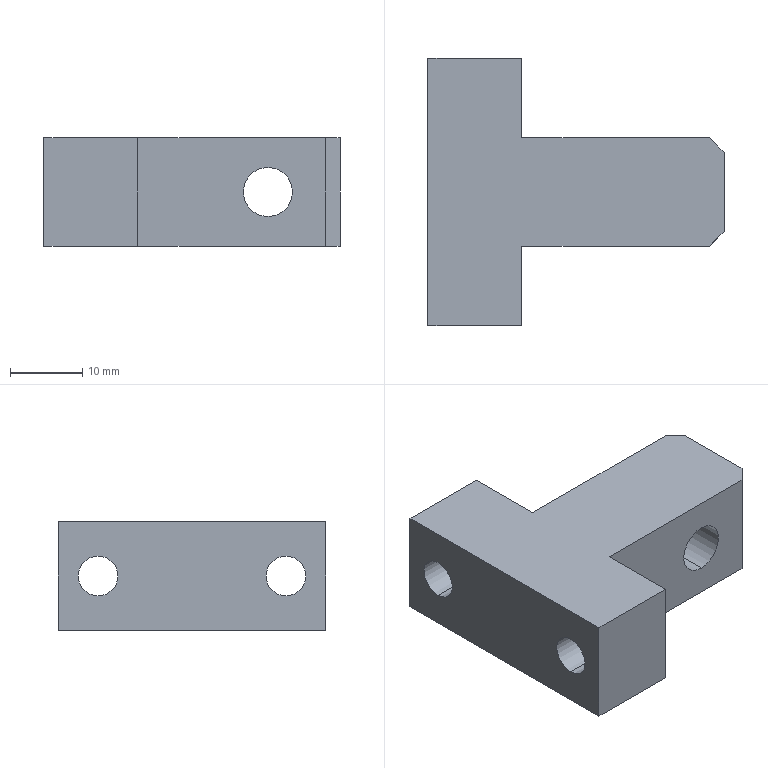Part | NX | features BREP 1 | 1 solid | 18 faces | box 41 x 37 x 15 mm | volume 12293 mm3 | plane 12 | cylinder 6 | commonest cylinder face diameters 5.5 x4 6.8 x2
STEP:
#1=CARTESIAN_POINT('',(-686.549,-298.31,10.25));
#2=VERTEX_POINT('',#1);
#3=CARTESIAN_POINT('',(-686.549,-298.31,4.75));
#4=VERTEX_POINT('',#3);
#5=CARTESIAN_POINT('',(-686.549,-298.31,7.5));
#6=DIRECTION('',(1.,0.,0.));
#7=DIRECTION('',(0.,0.,-1.));
#8=AXIS2_PLACEMENT_3D('',#5,#6,#7);
#9=CIRCLE('',#8,2.75);
#10=EDGE_CURVE('',#2,#4,#9,.T.);
#11=ORIENTED_EDGE('',*,*,#10,.F.);
#12=CARTESIAN_POINT('',(-673.549,-298.31,10.25));
#13=VERTEX_POINT('',#12);
#14=CARTESIAN_POINT('',(-686.549,-298.31,10.25));
#15=DIRECTION('',(1.,0.,0.));
#16=VECTOR('',#15,1000.);
#17=LINE('',#14,#16);
#18=EDGE_CURVE('',#2,#13,#17,.T.);
#19=ORIENTED_EDGE('',*,*,#18,.T.);
#20=CARTESIAN_POINT('',(-673.549,-298.31,4.75));
#21=VERTEX_POINT('',#20);
#22=CARTESIAN_POINT('',(-673.549,-298.31,7.5));
#23=DIRECTION('',(1.,0.,0.));
#24=DIRECTION('',(0.,0.,-1.));
#25=AXIS2_PLACEMENT_3D('',#22,#23,#24);
#26=CIRCLE('',#25,2.75);
#27=EDGE_CURVE('',#13,#21,#26,.T.);
#28=ORIENTED_EDGE('',*,*,#27,.T.);
#29=CARTESIAN_POINT('',(-686.549,-298.31,4.75));
#30=DIRECTION('',(1.,0.,0.));
#31=VECTOR('',#30,1000.);
#32=LINE('',#29,#31);
#33=EDGE_CURVE('',#4,#21,#32,.T.);
#34=ORIENTED_EDGE('',*,*,#33,.F.);
#35=EDGE_LOOP('',(#11,#19,#28,#34));
#36=FACE_BOUND('',#35,.T.);
#37=CARTESIAN_POINT('',(-686.549,-298.31,7.5));
#38=DIRECTION('',(1.,0.,0.));
#39=DIRECTION('',(0.,0.,-1.));
#40=AXIS2_PLACEMENT_3D('',#37,#38,#39);
#41=CYLINDRICAL_SURFACE('',#40,2.75);
#42=ADVANCED_FACE('',(#36),#41,.F.);
#43=CARTESIAN_POINT('',(-686.549,-324.31,10.25));
#44=VERTEX_POINT('',#43);
#45=CARTESIAN_POINT('',(-686.549,-324.31,4.75));
#46=VERTEX_POINT('',#45);
#47=CARTESIAN_POINT('',(-686.549,-324.31,7.5));
#48=DIRECTION('',(1.,0.,0.));
#49=DIRECTION('',(0.,0.,-1.));
#50=AXIS2_PLACEMENT_3D('',#47,#48,#49);
#51=CIRCLE('',#50,2.75);
#52=EDGE_CURVE('',#44,#46,#51,.T.);
#53=ORIENTED_EDGE('',*,*,#52,.F.);
#54=CARTESIAN_POINT('',(-673.549,-324.31,10.25));
#55=VERTEX_POINT('',#54);
#56=CARTESIAN_POINT('',(-686.549,-324.31,10.25));
#57=DIRECTION('',(1.,0.,0.));
#58=VECTOR('',#57,1000.);
#59=LINE('',#56,#58);
#60=EDGE_CURVE('',#44,#55,#59,.T.);
#61=ORIENTED_EDGE('',*,*,#60,.T.);
#62=CARTESIAN_POINT('',(-673.549,-324.31,4.75));
#63=VERTEX_POINT('',#62);
#64=CARTESIAN_POINT('',(-673.549,-324.31,7.5));
#65=DIRECTION('',(1.,0.,0.));
#66=DIRECTION('',(0.,0.,-1.));
#67=AXIS2_PLACEMENT_3D('',#64,#65,#66);
#68=CIRCLE('',#67,2.75);
#69=EDGE_CURVE('',#55,#63,#68,.T.);
#70=ORIENTED_EDGE('',*,*,#69,.T.);
#71=CARTESIAN_POINT('',(-686.549,-324.31,4.75));
#72=DIRECTION('',(1.,0.,0.));
#73=VECTOR('',#72,1000.);
#74=LINE('',#71,#73);
#75=EDGE_CURVE('',#46,#63,#74,.T.);
#76=ORIENTED_EDGE('',*,*,#75,.F.);
#77=EDGE_LOOP('',(#53,#61,#70,#76));
#78=FACE_BOUND('',#77,.T.);
#79=CARTESIAN_POINT('',(-686.549,-324.31,7.5));
#80=DIRECTION('',(1.,0.,0.));
#81=DIRECTION('',(0.,0.,-1.));
#82=AXIS2_PLACEMENT_3D('',#79,#80,#81);
#83=CYLINDRICAL_SURFACE('',#82,2.75);
#84=ADVANCED_FACE('',(#78),#83,.F.);
#85=CARTESIAN_POINT('',(-655.549,-303.81,10.9));
#86=VERTEX_POINT('',#85);
#87=CARTESIAN_POINT('',(-655.549,-303.81,4.1));
#88=VERTEX_POINT('',#87);
#89=CARTESIAN_POINT('',(-655.549,-303.81,7.5));
#90=DIRECTION('',(0.,-1.,0.));
#91=DIRECTION('',(1.,0.,0.));
#92=AXIS2_PLACEMENT_3D('',#89,#90,#91);
#93=CIRCLE('',#92,3.4);
#94=EDGE_CURVE('',#86,#88,#93,.T.);
#95=ORIENTED_EDGE('',*,*,#94,.F.);
#96=CARTESIAN_POINT('',(-655.549,-318.81,10.9));
#97=VERTEX_POINT('',#96);
#98=CARTESIAN_POINT('',(-655.549,-318.81,10.9));
#99=DIRECTION('',(0.,-1.,0.));
#100=VECTOR('',#99,1000.);
#101=LINE('',#98,#100);
#102=EDGE_CURVE('',#86,#97,#101,.T.);
#103=ORIENTED_EDGE('',*,*,#102,.T.);
#104=CARTESIAN_POINT('',(-655.549,-318.81,4.1));
#105=VERTEX_POINT('',#104);
#106=CARTESIAN_POINT('',(-655.549,-318.81,7.5));
#107=DIRECTION('',(0.,-1.,0.));
#108=DIRECTION('',(0.,0.,-1.));
#109=AXIS2_PLACEMENT_3D('',#106,#107,#108);
#110=CIRCLE('',#109,3.4);
#111=EDGE_CURVE('',#97,#105,#110,.T.);
#112=ORIENTED_EDGE('',*,*,#111,.T.);
#113=CARTESIAN_POINT('',(-655.549,-318.81,4.1));
#114=DIRECTION('',(0.,-1.,0.));
#115=VECTOR('',#114,1000.);
#116=LINE('',#113,#115);
#117=EDGE_CURVE('',#88,#105,#116,.T.);
#118=ORIENTED_EDGE('',*,*,#117,.F.);
#119=EDGE_LOOP('',(#95,#103,#112,#118));
#120=FACE_BOUND('',#119,.T.);
#121=CARTESIAN_POINT('',(-655.549,-318.81,7.5));
#122=DIRECTION('',(0.,-1.,0.));
#123=DIRECTION('',(0.,0.,-1.));
#124=AXIS2_PLACEMENT_3D('',#121,#122,#123);
#125=CYLINDRICAL_SURFACE('',#124,3.4);
#126=ADVANCED_FACE('',(#120),#125,.F.);
#127=CARTESIAN_POINT('',(-686.549,-292.81,0.));
#128=VERTEX_POINT('',#127);
#129=CARTESIAN_POINT('',(-686.549,-329.81,0.));
#130=VERTEX_POINT('',#129);
#131=CARTESIAN_POINT('',(-686.549,-292.81,0.));
#132=DIRECTION('',(0.,-1.,0.));
#133=VECTOR('',#132,1000.);
#134=LINE('',#131,#133);
#135=EDGE_CURVE('',#128,#130,#134,.T.);
#136=ORIENTED_EDGE('',*,*,#135,.T.);
#137=CARTESIAN_POINT('',(-686.549,-329.81,15.));
#138=VERTEX_POINT('',#137);
#139=CARTESIAN_POINT('',(-686.549,-329.81,15.));
#140=DIRECTION('',(0.,0.,-1.));
#141=VECTOR('',#140,1000.);
#142=LINE('',#139,#141);
#143=EDGE_CURVE('',#138,#130,#142,.T.);
#144=ORIENTED_EDGE('',*,*,#143,.F.);
#145=CARTESIAN_POINT('',(-686.549,-292.81,15.));
#146=VERTEX_POINT('',#145);
#147=CARTESIAN_POINT('',(-686.549,-292.81,15.));
#148=DIRECTION('',(0.,-1.,0.));
#149=VECTOR('',#148,1000.);
#150=LINE('',#147,#149);
#151=EDGE_CURVE('',#146,#138,#150,.T.);
#152=ORIENTED_EDGE('',*,*,#151,.F.);
#153=CARTESIAN_POINT('',(-686.549,-292.81,15.));
#154=DIRECTION('',(0.,0.,-1.));
#155=VECTOR('',#154,1000.);
#156=LINE('',#153,#155);
#157=EDGE_CURVE('',#146,#128,#156,.T.);
#158=ORIENTED_EDGE('',*,*,#157,.T.);
#159=EDGE_LOOP('',(#136,#144,#152,#158));
#160=FACE_BOUND('',#159,.T.);
#161=CARTESIAN_POINT('',(-686.549,-298.31,7.5));
#162=DIRECTION('',(1.,0.,0.));
#163=DIRECTION('',(0.,0.,-1.));
#164=AXIS2_PLACEMENT_3D('',#161,#162,#163);
#165=CIRCLE('',#164,2.75);
#166=EDGE_CURVE('',#4,#2,#165,.T.);
#167=ORIENTED_EDGE('',*,*,#166,.T.);
#168=ORIENTED_EDGE('',*,*,#10,.T.);
#169=EDGE_LOOP('',(#167,#168));
#170=FACE_BOUND('',#169,.T.);
#171=CARTESIAN_POINT('',(-686.549,-324.31,7.5));
#172=DIRECTION('',(1.,0.,0.));
#173=DIRECTION('',(0.,0.,-1.));
#174=AXIS2_PLACEMENT_3D('',#171,#172,#173);
#175=CIRCLE('',#174,2.75);
#176=EDGE_CURVE('',#46,#44,#175,.T.);
#177=ORIENTED_EDGE('',*,*,#176,.T.);
#178=ORIENTED_EDGE('',*,*,#52,.T.);
#179=EDGE_LOOP('',(#177,#178));
#180=FACE_BOUND('',#179,.T.);
#181=CARTESIAN_POINT('',(-686.549,-292.81,15.));
#182=DIRECTION('',(1.,0.,0.));
#183=DIRECTION('',(0.,1.,0.));
#184=AXIS2_PLACEMENT_3D('',#181,#182,#183);
#185=PLANE('',#184);
#186=ADVANCED_FACE('',(#160,#170,#180),#185,.F.);
#187=CARTESIAN_POINT('',(-673.549,-329.81,0.));
#188=VERTEX_POINT('',#187);
#189=CARTESIAN_POINT('',(-686.549,-329.81,0.));
#190=DIRECTION('',(1.,0.,0.));
#191=VECTOR('',#190,1000.);
#192=LINE('',#189,#191);
#193=EDGE_CURVE('',#130,#188,#192,.T.);
#194=ORIENTED_EDGE('',*,*,#193,.T.);
#195=CARTESIAN_POINT('',(-673.549,-329.81,15.));
#196=VERTEX_POINT('',#195);
#197=CARTESIAN_POINT('',(-673.549,-329.81,15.));
#198=DIRECTION('',(0.,0.,-1.));
#199=VECTOR('',#198,1000.);
#200=LINE('',#197,#199);
#201=EDGE_CURVE('',#196,#188,#200,.T.);
#202=ORIENTED_EDGE('',*,*,#201,.F.);
#203=CARTESIAN_POINT('',(-686.549,-329.81,15.));
#204=DIRECTION('',(1.,0.,0.));
#205=VECTOR('',#204,1000.);
#206=LINE('',#203,#205);
#207=EDGE_CURVE('',#138,#196,#206,.T.);
#208=ORIENTED_EDGE('',*,*,#207,.F.);
#209=ORIENTED_EDGE('',*,*,#143,.T.);
#210=EDGE_LOOP('',(#194,#202,#208,#209));
#211=FACE_BOUND('',#210,.T.);
#212=CARTESIAN_POINT('',(-686.549,-329.81,15.));
#213=DIRECTION('',(0.,1.,0.));
#214=DIRECTION('',(1.,0.,0.));
#215=AXIS2_PLACEMENT_3D('',#212,#213,#214);
#216=PLANE('',#215);
#217=ADVANCED_FACE('',(#211),#216,.F.);
#218=CARTESIAN_POINT('',(-673.549,-318.81,0.));
#219=VERTEX_POINT('',#218);
#220=CARTESIAN_POINT('',(-673.549,-318.81,0.));
#221=DIRECTION('',(0.,1.,0.));
#222=VECTOR('',#221,1000.);
#223=LINE('',#220,#222);
#224=EDGE_CURVE('',#188,#219,#223,.T.);
#225=ORIENTED_EDGE('',*,*,#224,.T.);
#226=CARTESIAN_POINT('',(-673.549,-318.81,15.));
#227=VERTEX_POINT('',#226);
#228=CARTESIAN_POINT('',(-673.549,-318.81,15.));
#229=DIRECTION('',(0.,0.,-1.));
#230=VECTOR('',#229,1000.);
#231=LINE('',#228,#230);
#232=EDGE_CURVE('',#227,#219,#231,.T.);
#233=ORIENTED_EDGE('',*,*,#232,.F.);
#234=CARTESIAN_POINT('',(-673.549,-318.81,15.));
#235=DIRECTION('',(0.,1.,0.));
#236=VECTOR('',#235,1000.);
#237=LINE('',#234,#236);
#238=EDGE_CURVE('',#196,#227,#237,.T.);
#239=ORIENTED_EDGE('',*,*,#238,.F.);
#240=ORIENTED_EDGE('',*,*,#201,.T.);
#241=EDGE_LOOP('',(#225,#233,#239,#240));
#242=FACE_BOUND('',#241,.T.);
#243=CARTESIAN_POINT('',(-673.549,-324.31,7.5));
#244=DIRECTION('',(1.,0.,0.));
#245=DIRECTION('',(0.,0.,-1.));
#246=AXIS2_PLACEMENT_3D('',#243,#244,#245);
#247=CIRCLE('',#246,2.75);
#248=EDGE_CURVE('',#63,#55,#247,.T.);
#249=ORIENTED_EDGE('',*,*,#248,.F.);
#250=ORIENTED_EDGE('',*,*,#69,.F.);
#251=EDGE_LOOP('',(#249,#250));
#252=FACE_BOUND('',#251,.T.);
#253=CARTESIAN_POINT('',(-673.549,-318.81,15.));
#254=DIRECTION('',(-1.,0.,0.));
#255=DIRECTION('',(0.,0.,1.));
#256=AXIS2_PLACEMENT_3D('',#253,#254,#255);
#257=PLANE('',#256);
#258=ADVANCED_FACE('',(#242,#252),#257,.F.);
#259=CARTESIAN_POINT('',(-647.549,-318.81,0.));
#260=VERTEX_POINT('',#259);
#261=CARTESIAN_POINT('',(-673.549,-318.81,0.));
#262=DIRECTION('',(1.,0.,0.));
#263=VECTOR('',#262,1000.);
#264=LINE('',#261,#263);
#265=EDGE_CURVE('',#219,#260,#264,.T.);
#266=ORIENTED_EDGE('',*,*,#265,.T.);
#267=CARTESIAN_POINT('',(-647.549,-318.81,15.));
#268=VERTEX_POINT('',#267);
#269=CARTESIAN_POINT('',(-647.549,-318.81,15.));
#270=DIRECTION('',(0.,0.,1.));
#271=VECTOR('',#270,1000.);
#272=LINE('',#269,#271);
#273=EDGE_CURVE('',#260,#268,#272,.T.);
#274=ORIENTED_EDGE('',*,*,#273,.T.);
#275=CARTESIAN_POINT('',(-673.549,-318.81,15.));
#276=DIRECTION('',(1.,0.,0.));
#277=VECTOR('',#276,1000.);
#278=LINE('',#275,#277);
#279=EDGE_CURVE('',#227,#268,#278,.T.);
#280=ORIENTED_EDGE('',*,*,#279,.F.);
#281=ORIENTED_EDGE('',*,*,#232,.T.);
#282=EDGE_LOOP('',(#266,#274,#280,#281));
#283=FACE_BOUND('',#282,.T.);
#284=CARTESIAN_POINT('',(-655.549,-318.81,7.5));
#285=DIRECTION('',(0.,-1.,0.));
#286=DIRECTION('',(0.,0.,-1.));
#287=AXIS2_PLACEMENT_3D('',#284,#285,#286);
#288=CIRCLE('',#287,3.4);
#289=EDGE_CURVE('',#105,#97,#288,.T.);
#290=ORIENTED_EDGE('',*,*,#289,.F.);
#291=ORIENTED_EDGE('',*,*,#111,.F.);
#292=EDGE_LOOP('',(#290,#291));
#293=FACE_BOUND('',#292,.T.);
#294=CARTESIAN_POINT('',(-673.549,-318.81,15.));
#295=DIRECTION('',(0.,1.,0.));
#296=DIRECTION('',(1.,0.,0.));
#297=AXIS2_PLACEMENT_3D('',#294,#295,#296);
#298=PLANE('',#297);
#299=ADVANCED_FACE('',(#283,#293),#298,.F.);
#300=CARTESIAN_POINT('',(-645.549,-316.81,0.));
#301=VERTEX_POINT('',#300);
#302=CARTESIAN_POINT('',(-645.549,-305.81,0.));
#303=VERTEX_POINT('',#302);
#304=CARTESIAN_POINT('',(-645.549,-303.81,0.));
#305=DIRECTION('',(0.,1.,0.));
#306=VECTOR('',#305,1000.);
#307=LINE('',#304,#306);
#308=EDGE_CURVE('',#301,#303,#307,.T.);
#309=ORIENTED_EDGE('',*,*,#308,.T.);
#310=CARTESIAN_POINT('',(-645.549,-305.81,15.));
#311=VERTEX_POINT('',#310);
#312=CARTESIAN_POINT('',(-645.549,-305.81,15.));
#313=DIRECTION('',(0.,0.,1.));
#314=VECTOR('',#313,1000.);
#315=LINE('',#312,#314);
#316=EDGE_CURVE('',#303,#311,#315,.T.);
#317=ORIENTED_EDGE('',*,*,#316,.T.);
#318=CARTESIAN_POINT('',(-645.549,-316.81,15.));
#319=VERTEX_POINT('',#318);
#320=CARTESIAN_POINT('',(-645.549,-303.81,15.));
#321=DIRECTION('',(0.,1.,0.));
#322=VECTOR('',#321,1000.);
#323=LINE('',#320,#322);
#324=EDGE_CURVE('',#319,#311,#323,.T.);
#325=ORIENTED_EDGE('',*,*,#324,.F.);
#326=CARTESIAN_POINT('',(-645.549,-316.81,15.));
#327=DIRECTION('',(0.,0.,-1.));
#328=VECTOR('',#327,1000.);
#329=LINE('',#326,#328);
#330=EDGE_CURVE('',#319,#301,#329,.T.);
#331=ORIENTED_EDGE('',*,*,#330,.T.);
#332=EDGE_LOOP('',(#309,#317,#325,#331));
#333=FACE_BOUND('',#332,.T.);
#334=CARTESIAN_POINT('',(-645.549,-303.81,15.));
#335=DIRECTION('',(-1.,0.,0.));
#336=DIRECTION('',(0.,0.,1.));
#337=AXIS2_PLACEMENT_3D('',#334,#335,#336);
#338=PLANE('',#337);
#339=ADVANCED_FACE('',(#333),#338,.F.);
#340=CARTESIAN_POINT('',(-647.549,-303.81,15.));
#341=VERTEX_POINT('',#340);
#342=CARTESIAN_POINT('',(-673.549,-303.81,15.));
#343=VERTEX_POINT('',#342);
#344=CARTESIAN_POINT('',(-673.549,-303.81,15.));
#345=DIRECTION('',(-1.,0.,0.));
#346=VECTOR('',#345,1000.);
#347=LINE('',#344,#346);
#348=EDGE_CURVE('',#341,#343,#347,.T.);
#349=ORIENTED_EDGE('',*,*,#348,.F.);
#350=CARTESIAN_POINT('',(-647.549,-303.81,0.));
#351=VERTEX_POINT('',#350);
#352=CARTESIAN_POINT('',(-647.549,-303.81,15.));
#353=DIRECTION('',(0.,0.,-1.));
#354=VECTOR('',#353,1000.);
#355=LINE('',#352,#354);
#356=EDGE_CURVE('',#341,#351,#355,.T.);
#357=ORIENTED_EDGE('',*,*,#356,.T.);
#358=CARTESIAN_POINT('',(-673.549,-303.81,0.));
#359=VERTEX_POINT('',#358);
#360=CARTESIAN_POINT('',(-673.549,-303.81,0.));
#361=DIRECTION('',(-1.,0.,0.));
#362=VECTOR('',#361,1000.);
#363=LINE('',#360,#362);
#364=EDGE_CURVE('',#351,#359,#363,.T.);
#365=ORIENTED_EDGE('',*,*,#364,.T.);
#366=CARTESIAN_POINT('',(-673.549,-303.81,15.));
#367=DIRECTION('',(0.,0.,-1.));
#368=VECTOR('',#367,1000.);
#369=LINE('',#366,#368);
#370=EDGE_CURVE('',#343,#359,#369,.T.);
#371=ORIENTED_EDGE('',*,*,#370,.F.);
#372=EDGE_LOOP('',(#349,#357,#365,#371));
#373=FACE_BOUND('',#372,.T.);
#374=CARTESIAN_POINT('',(-655.549,-303.81,7.5));
#375=DIRECTION('',(0.,-1.,0.));
#376=DIRECTION('',(1.,0.,0.));
#377=AXIS2_PLACEMENT_3D('',#374,#375,#376);
#378=CIRCLE('',#377,3.4);
#379=EDGE_CURVE('',#88,#86,#378,.T.);
#380=ORIENTED_EDGE('',*,*,#379,.T.);
#381=ORIENTED_EDGE('',*,*,#94,.T.);
#382=EDGE_LOOP('',(#380,#381));
#383=FACE_BOUND('',#382,.T.);
#384=CARTESIAN_POINT('',(-673.549,-303.81,15.));
#385=DIRECTION('',(0.,-1.,0.));
#386=DIRECTION('',(0.,0.,-1.));
#387=AXIS2_PLACEMENT_3D('',#384,#385,#386);
#388=PLANE('',#387);
#389=ADVANCED_FACE('',(#373,#383),#388,.F.);
#390=CARTESIAN_POINT('',(-673.549,-292.81,0.));
#391=VERTEX_POINT('',#390);
#392=CARTESIAN_POINT('',(-673.549,-292.81,0.));
#393=DIRECTION('',(0.,1.,0.));
#394=VECTOR('',#393,1000.);
#395=LINE('',#392,#394);
#396=EDGE_CURVE('',#359,#391,#395,.T.);
#397=ORIENTED_EDGE('',*,*,#396,.T.);
#398=CARTESIAN_POINT('',(-673.549,-292.81,15.));
#399=VERTEX_POINT('',#398);
#400=CARTESIAN_POINT('',(-673.549,-292.81,15.));
#401=DIRECTION('',(0.,0.,-1.));
#402=VECTOR('',#401,1000.);
#403=LINE('',#400,#402);
#404=EDGE_CURVE('',#399,#391,#403,.T.);
#405=ORIENTED_EDGE('',*,*,#404,.F.);
#406=CARTESIAN_POINT('',(-673.549,-292.81,15.));
#407=DIRECTION('',(0.,1.,0.));
#408=VECTOR('',#407,1000.);
#409=LINE('',#406,#408);
#410=EDGE_CURVE('',#343,#399,#409,.T.);
#411=ORIENTED_EDGE('',*,*,#410,.F.);
#412=ORIENTED_EDGE('',*,*,#370,.T.);
#413=EDGE_LOOP('',(#397,#405,#411,#412));
#414=FACE_BOUND('',#413,.T.);
#415=CARTESIAN_POINT('',(-673.549,-298.31,7.5));
#416=DIRECTION('',(1.,0.,0.));
#417=DIRECTION('',(0.,0.,-1.));
#418=AXIS2_PLACEMENT_3D('',#415,#416,#417);
#419=CIRCLE('',#418,2.75);
#420=EDGE_CURVE('',#21,#13,#419,.T.);
#421=ORIENTED_EDGE('',*,*,#420,.F.);
#422=ORIENTED_EDGE('',*,*,#27,.F.);
#423=EDGE_LOOP('',(#421,#422));
#424=FACE_BOUND('',#423,.T.);
#425=CARTESIAN_POINT('',(-673.549,-292.81,15.));
#426=DIRECTION('',(-1.,0.,0.));
#427=DIRECTION('',(0.,0.,1.));
#428=AXIS2_PLACEMENT_3D('',#425,#426,#427);
#429=PLANE('',#428);
#430=ADVANCED_FACE('',(#414,#424),#429,.F.);
#431=CARTESIAN_POINT('',(-686.549,-292.81,0.));
#432=DIRECTION('',(-1.,0.,0.));
#433=VECTOR('',#432,1000.);
#434=LINE('',#431,#433);
#435=EDGE_CURVE('',#391,#128,#434,.T.);
#436=ORIENTED_EDGE('',*,*,#435,.T.);
#437=ORIENTED_EDGE('',*,*,#157,.F.);
#438=CARTESIAN_POINT('',(-686.549,-292.81,15.));
#439=DIRECTION('',(-1.,0.,0.));
#440=VECTOR('',#439,1000.);
#441=LINE('',#438,#440);
#442=EDGE_CURVE('',#399,#146,#441,.T.);
#443=ORIENTED_EDGE('',*,*,#442,.F.);
#444=ORIENTED_EDGE('',*,*,#404,.T.);
#445=EDGE_LOOP('',(#436,#437,#443,#444));
#446=FACE_BOUND('',#445,.T.);
#447=CARTESIAN_POINT('',(-686.549,-292.81,15.));
#448=DIRECTION('',(0.,-1.,0.));
#449=DIRECTION('',(0.,0.,-1.));
#450=AXIS2_PLACEMENT_3D('',#447,#448,#449);
#451=PLANE('',#450);
#452=ADVANCED_FACE('',(#446),#451,.F.);
#453=ORIENTED_EDGE('',*,*,#324,.T.);
#454=CARTESIAN_POINT('',(-654.049,-297.31,15.));
#455=DIRECTION('',(-0.7071,0.7071,0.));
#456=VECTOR('',#455,1000.);
#457=LINE('',#454,#456);
#458=EDGE_CURVE('',#311,#341,#457,.T.);
#459=ORIENTED_EDGE('',*,*,#458,.T.);
#460=ORIENTED_EDGE('',*,*,#348,.T.);
#461=ORIENTED_EDGE('',*,*,#410,.T.);
#462=ORIENTED_EDGE('',*,*,#442,.T.);
#463=ORIENTED_EDGE('',*,*,#151,.T.);
#464=ORIENTED_EDGE('',*,*,#207,.T.);
#465=ORIENTED_EDGE('',*,*,#238,.T.);
#466=ORIENTED_EDGE('',*,*,#279,.T.);
#467=CARTESIAN_POINT('',(-672.549,-343.81,15.));
#468=DIRECTION('',(0.7071,0.7071,0.));
#469=VECTOR('',#468,1000.);
#470=LINE('',#467,#469);
#471=EDGE_CURVE('',#268,#319,#470,.T.);
#472=ORIENTED_EDGE('',*,*,#471,.T.);
#473=EDGE_LOOP('',(#453,#459,#460,#461,#462,#463,#464,#465,#466,#472));
#474=FACE_BOUND('',#473,.T.);
#475=CARTESIAN_POINT('',(-686.549,-329.81,15.));
#476=DIRECTION('',(0.,0.,1.));
#477=DIRECTION('',(1.,0.,0.));
#478=AXIS2_PLACEMENT_3D('',#475,#476,#477);
#479=PLANE('',#478);
#480=ADVANCED_FACE('',(#474),#479,.T.);
#481=ORIENTED_EDGE('',*,*,#364,.F.);
#482=CARTESIAN_POINT('',(-647.549,-303.81,0.));
#483=DIRECTION('',(0.7071,-0.7071,0.));
#484=VECTOR('',#483,1000.);
#485=LINE('',#482,#484);
#486=EDGE_CURVE('',#351,#303,#485,.T.);
#487=ORIENTED_EDGE('',*,*,#486,.T.);
#488=ORIENTED_EDGE('',*,*,#308,.F.);
#489=CARTESIAN_POINT('',(-645.549,-316.81,0.));
#490=DIRECTION('',(-0.7071,-0.7071,0.));
#491=VECTOR('',#490,1000.);
#492=LINE('',#489,#491);
#493=EDGE_CURVE('',#301,#260,#492,.T.);
#494=ORIENTED_EDGE('',*,*,#493,.T.);
#495=ORIENTED_EDGE('',*,*,#265,.F.);
#496=ORIENTED_EDGE('',*,*,#224,.F.);
#497=ORIENTED_EDGE('',*,*,#193,.F.);
#498=ORIENTED_EDGE('',*,*,#135,.F.);
#499=ORIENTED_EDGE('',*,*,#435,.F.);
#500=ORIENTED_EDGE('',*,*,#396,.F.);
#501=EDGE_LOOP('',(#481,#487,#488,#494,#495,#496,#497,#498,#499,#500));
#502=FACE_BOUND('',#501,.T.);
#503=CARTESIAN_POINT('',(-686.549,-329.81,0.));
#504=DIRECTION('',(0.,0.,1.));
#505=DIRECTION('',(1.,0.,0.));
#506=AXIS2_PLACEMENT_3D('',#503,#504,#505);
#507=PLANE('',#506);
#508=ADVANCED_FACE('',(#502),#507,.F.);
#509=ORIENTED_EDGE('',*,*,#102,.F.);
#510=ORIENTED_EDGE('',*,*,#379,.F.);
#511=ORIENTED_EDGE('',*,*,#117,.T.);
#512=ORIENTED_EDGE('',*,*,#289,.T.);
#513=EDGE_LOOP('',(#509,#510,#511,#512));
#514=FACE_BOUND('',#513,.T.);
#515=CARTESIAN_POINT('',(-655.549,-318.81,7.5));
#516=DIRECTION('',(0.,-1.,0.));
#517=DIRECTION('',(0.,0.,-1.));
#518=AXIS2_PLACEMENT_3D('',#515,#516,#517);
#519=CYLINDRICAL_SURFACE('',#518,3.4);
#520=ADVANCED_FACE('',(#514),#519,.F.);
#521=ORIENTED_EDGE('',*,*,#60,.F.);
#522=ORIENTED_EDGE('',*,*,#176,.F.);
#523=ORIENTED_EDGE('',*,*,#75,.T.);
#524=ORIENTED_EDGE('',*,*,#248,.T.);
#525=EDGE_LOOP('',(#521,#522,#523,#524));
#526=FACE_BOUND('',#525,.T.);
#527=CARTESIAN_POINT('',(-686.549,-324.31,7.5));
#528=DIRECTION('',(1.,0.,0.));
#529=DIRECTION('',(0.,0.,-1.));
#530=AXIS2_PLACEMENT_3D('',#527,#528,#529);
#531=CYLINDRICAL_SURFACE('',#530,2.75);
#532=ADVANCED_FACE('',(#526),#531,.F.);
#533=ORIENTED_EDGE('',*,*,#18,.F.);
#534=ORIENTED_EDGE('',*,*,#166,.F.);
#535=ORIENTED_EDGE('',*,*,#33,.T.);
#536=ORIENTED_EDGE('',*,*,#420,.T.);
#537=EDGE_LOOP('',(#533,#534,#535,#536));
#538=FACE_BOUND('',#537,.T.);
#539=CARTESIAN_POINT('',(-686.549,-298.31,7.5));
#540=DIRECTION('',(1.,0.,0.));
#541=DIRECTION('',(0.,0.,-1.));
#542=AXIS2_PLACEMENT_3D('',#539,#540,#541);
#543=CYLINDRICAL_SURFACE('',#542,2.75);
#544=ADVANCED_FACE('',(#538),#543,.F.);
#545=ORIENTED_EDGE('',*,*,#458,.F.);
#546=ORIENTED_EDGE('',*,*,#316,.F.);
#547=ORIENTED_EDGE('',*,*,#486,.F.);
#548=ORIENTED_EDGE('',*,*,#356,.F.);
#549=EDGE_LOOP('',(#545,#546,#547,#548));
#550=FACE_BOUND('',#549,.T.);
#551=CARTESIAN_POINT('',(-647.549,-303.81,15.));
#552=DIRECTION('',(-0.7071,-0.7071,0.));
#553=DIRECTION('',(-0.7071,0.7071,0.));
#554=AXIS2_PLACEMENT_3D('',#551,#552,#553);
#555=PLANE('',#554);
#556=ADVANCED_FACE('',(#550),#555,.F.);
#557=ORIENTED_EDGE('',*,*,#471,.F.);
#558=ORIENTED_EDGE('',*,*,#273,.F.);
#559=ORIENTED_EDGE('',*,*,#493,.F.);
#560=ORIENTED_EDGE('',*,*,#330,.F.);
#561=EDGE_LOOP('',(#557,#558,#559,#560));
#562=FACE_BOUND('',#561,.T.);
#563=CARTESIAN_POINT('',(-645.549,-316.81,15.));
#564=DIRECTION('',(-0.7071,0.7071,0.));
#565=DIRECTION('',(0.,0.,1.));
#566=AXIS2_PLACEMENT_3D('',#563,#564,#565);
#567=PLANE('',#566);
#568=ADVANCED_FACE('',(#562),#567,.F.);
#569=CLOSED_SHELL('',(#42,#84,#126,#186,#217,#258,#299,#339,#389,#430,#452,#480,#508,#520,#532,#544,#556,#568));
#570=MANIFOLD_SOLID_BREP('',#569);
#571=(LENGTH_UNIT()NAMED_UNIT(*)SI_UNIT(.MILLI.,.METRE.));
#572=UNCERTAINTY_MEASURE_WITH_UNIT(LENGTH_MEASURE(0.00001),#571,'','');
#573=(NAMED_UNIT(*)PLANE_ANGLE_UNIT()SI_UNIT($,.RADIAN.));
#574=(NAMED_UNIT(*)SI_UNIT($,.STERADIAN.)SOLID_ANGLE_UNIT());
#575=(GEOMETRIC_REPRESENTATION_CONTEXT(3)GLOBAL_UNCERTAINTY_ASSIGNED_CONTEXT((#572))GLOBAL_UNIT_ASSIGNED_CONTEXT((#571,#573,#574))REPRESENTATION_CONTEXT('',''));
#576=ADVANCED_BREP_SHAPE_REPRESENTATION('',(#570),#575);